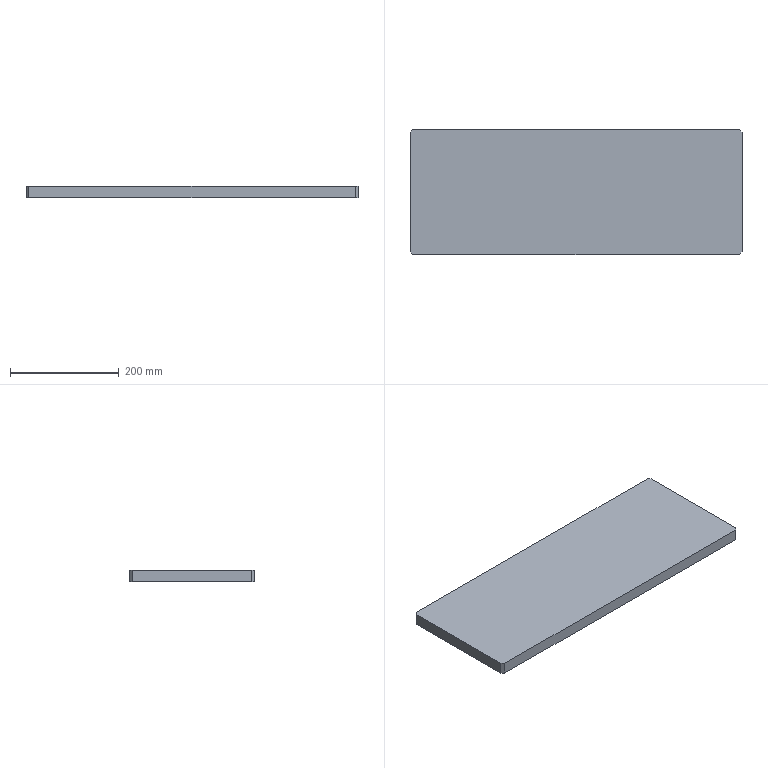Part | SolidWorks | features Chamfer 1, Extrusion 1 | 1 solid | 10 faces | box 610 x 230 x 22 mm | volume 3085500 mm3 | plane 10
STEP:
#1=CARTESIAN_POINT('',(558.381,212.028,22.));
#2=VERTEX_POINT('',#1);
#3=CARTESIAN_POINT('',(-41.619,212.028,22.));
#4=VERTEX_POINT('',#3);
#5=CARTESIAN_POINT('',(-46.619,212.028,22.));
#6=DIRECTION('',(-1.,0.,0.));
#7=VECTOR('',#6,1000.);
#8=LINE('',#5,#7);
#9=EDGE_CURVE('',#2,#4,#8,.T.);
#10=ORIENTED_EDGE('',*,*,#9,.F.);
#11=CARTESIAN_POINT('',(558.381,212.028,0.));
#12=VERTEX_POINT('',#11);
#13=CARTESIAN_POINT('',(558.381,212.028,22.));
#14=DIRECTION('',(0.,0.,-1.));
#15=VECTOR('',#14,1000.);
#16=LINE('',#13,#15);
#17=EDGE_CURVE('',#2,#12,#16,.T.);
#18=ORIENTED_EDGE('',*,*,#17,.T.);
#19=CARTESIAN_POINT('',(-41.619,212.028,0.));
#20=VERTEX_POINT('',#19);
#21=CARTESIAN_POINT('',(-46.619,212.028,0.));
#22=DIRECTION('',(-1.,0.,0.));
#23=VECTOR('',#22,1000.);
#24=LINE('',#21,#23);
#25=EDGE_CURVE('',#12,#20,#24,.T.);
#26=ORIENTED_EDGE('',*,*,#25,.T.);
#27=CARTESIAN_POINT('',(-41.619,212.028,22.));
#28=DIRECTION('',(0.,0.,1.));
#29=VECTOR('',#28,1000.);
#30=LINE('',#27,#29);
#31=EDGE_CURVE('',#20,#4,#30,.T.);
#32=ORIENTED_EDGE('',*,*,#31,.T.);
#33=EDGE_LOOP('',(#10,#18,#26,#32));
#34=FACE_OUTER_BOUND('',#33,.T.);
#35=CARTESIAN_POINT('',(-46.619,212.028,22.));
#36=DIRECTION('',(0.,-1.,0.));
#37=DIRECTION('',(0.,0.,-1.));
#38=AXIS2_PLACEMENT_3D('',#35,#36,#37);
#39=PLANE('',#38);
#40=ADVANCED_FACE('',(#34),#39,.F.);
#41=CARTESIAN_POINT('',(-46.619,207.028,0.));
#42=VERTEX_POINT('',#41);
#43=CARTESIAN_POINT('',(-46.619,-12.972,0.));
#44=VERTEX_POINT('',#43);
#45=CARTESIAN_POINT('',(-46.619,212.028,0.));
#46=DIRECTION('',(0.,-1.,0.));
#47=VECTOR('',#46,1000.);
#48=LINE('',#45,#47);
#49=EDGE_CURVE('',#42,#44,#48,.T.);
#50=ORIENTED_EDGE('',*,*,#49,.T.);
#51=CARTESIAN_POINT('',(-46.619,-12.972,22.));
#52=VERTEX_POINT('',#51);
#53=CARTESIAN_POINT('',(-46.619,-12.972,22.));
#54=DIRECTION('',(0.,0.,1.));
#55=VECTOR('',#54,1000.);
#56=LINE('',#53,#55);
#57=EDGE_CURVE('',#44,#52,#56,.T.);
#58=ORIENTED_EDGE('',*,*,#57,.T.);
#59=CARTESIAN_POINT('',(-46.619,207.028,22.));
#60=VERTEX_POINT('',#59);
#61=CARTESIAN_POINT('',(-46.619,212.028,22.));
#62=DIRECTION('',(0.,-1.,0.));
#63=VECTOR('',#62,1000.);
#64=LINE('',#61,#63);
#65=EDGE_CURVE('',#60,#52,#64,.T.);
#66=ORIENTED_EDGE('',*,*,#65,.F.);
#67=CARTESIAN_POINT('',(-46.619,207.028,22.));
#68=DIRECTION('',(0.,0.,-1.));
#69=VECTOR('',#68,1000.);
#70=LINE('',#67,#69);
#71=EDGE_CURVE('',#60,#42,#70,.T.);
#72=ORIENTED_EDGE('',*,*,#71,.T.);
#73=EDGE_LOOP('',(#50,#58,#66,#72));
#74=FACE_OUTER_BOUND('',#73,.T.);
#75=CARTESIAN_POINT('',(-46.619,212.028,22.));
#76=DIRECTION('',(1.,0.,0.));
#77=DIRECTION('',(0.,1.,0.));
#78=AXIS2_PLACEMENT_3D('',#75,#76,#77);
#79=PLANE('',#78);
#80=ADVANCED_FACE('',(#74),#79,.F.);
#81=CARTESIAN_POINT('',(-41.619,-17.972,0.));
#82=VERTEX_POINT('',#81);
#83=CARTESIAN_POINT('',(558.381,-17.972,0.));
#84=VERTEX_POINT('',#83);
#85=CARTESIAN_POINT('',(563.381,-17.972,0.));
#86=DIRECTION('',(1.,0.,0.));
#87=VECTOR('',#86,1000.);
#88=LINE('',#85,#87);
#89=EDGE_CURVE('',#82,#84,#88,.T.);
#90=ORIENTED_EDGE('',*,*,#89,.T.);
#91=CARTESIAN_POINT('',(558.381,-17.972,22.));
#92=VERTEX_POINT('',#91);
#93=CARTESIAN_POINT('',(558.381,-17.972,22.));
#94=DIRECTION('',(0.,0.,1.));
#95=VECTOR('',#94,1000.);
#96=LINE('',#93,#95);
#97=EDGE_CURVE('',#84,#92,#96,.T.);
#98=ORIENTED_EDGE('',*,*,#97,.T.);
#99=CARTESIAN_POINT('',(-41.619,-17.972,22.));
#100=VERTEX_POINT('',#99);
#101=CARTESIAN_POINT('',(563.381,-17.972,22.));
#102=DIRECTION('',(1.,0.,0.));
#103=VECTOR('',#102,1000.);
#104=LINE('',#101,#103);
#105=EDGE_CURVE('',#100,#92,#104,.T.);
#106=ORIENTED_EDGE('',*,*,#105,.F.);
#107=CARTESIAN_POINT('',(-41.619,-17.972,22.));
#108=DIRECTION('',(0.,0.,-1.));
#109=VECTOR('',#108,1000.);
#110=LINE('',#107,#109);
#111=EDGE_CURVE('',#100,#82,#110,.T.);
#112=ORIENTED_EDGE('',*,*,#111,.T.);
#113=EDGE_LOOP('',(#90,#98,#106,#112));
#114=FACE_OUTER_BOUND('',#113,.T.);
#115=CARTESIAN_POINT('',(563.381,-17.972,22.));
#116=DIRECTION('',(0.,1.,0.));
#117=DIRECTION('',(-1.,0.,0.));
#118=AXIS2_PLACEMENT_3D('',#115,#116,#117);
#119=PLANE('',#118);
#120=ADVANCED_FACE('',(#114),#119,.F.);
#121=CARTESIAN_POINT('',(563.381,-12.972,22.));
#122=VERTEX_POINT('',#121);
#123=CARTESIAN_POINT('',(563.381,207.028,22.));
#124=VERTEX_POINT('',#123);
#125=CARTESIAN_POINT('',(563.381,212.028,22.));
#126=DIRECTION('',(0.,1.,0.));
#127=VECTOR('',#126,1000.);
#128=LINE('',#125,#127);
#129=EDGE_CURVE('',#122,#124,#128,.T.);
#130=ORIENTED_EDGE('',*,*,#129,.F.);
#131=CARTESIAN_POINT('',(563.381,-12.972,0.));
#132=VERTEX_POINT('',#131);
#133=CARTESIAN_POINT('',(563.381,-12.972,22.));
#134=DIRECTION('',(0.,0.,-1.));
#135=VECTOR('',#134,1000.);
#136=LINE('',#133,#135);
#137=EDGE_CURVE('',#122,#132,#136,.T.);
#138=ORIENTED_EDGE('',*,*,#137,.T.);
#139=CARTESIAN_POINT('',(563.381,207.028,0.));
#140=VERTEX_POINT('',#139);
#141=CARTESIAN_POINT('',(563.381,212.028,0.));
#142=DIRECTION('',(0.,1.,0.));
#143=VECTOR('',#142,1000.);
#144=LINE('',#141,#143);
#145=EDGE_CURVE('',#132,#140,#144,.T.);
#146=ORIENTED_EDGE('',*,*,#145,.T.);
#147=CARTESIAN_POINT('',(563.381,207.028,22.));
#148=DIRECTION('',(0.,0.,1.));
#149=VECTOR('',#148,1000.);
#150=LINE('',#147,#149);
#151=EDGE_CURVE('',#140,#124,#150,.T.);
#152=ORIENTED_EDGE('',*,*,#151,.T.);
#153=EDGE_LOOP('',(#130,#138,#146,#152));
#154=FACE_OUTER_BOUND('',#153,.T.);
#155=CARTESIAN_POINT('',(563.381,212.028,22.));
#156=DIRECTION('',(-1.,0.,0.));
#157=DIRECTION('',(0.,0.,1.));
#158=AXIS2_PLACEMENT_3D('',#155,#156,#157);
#159=PLANE('',#158);
#160=ADVANCED_FACE('',(#154),#159,.F.);
#161=ORIENTED_EDGE('',*,*,#105,.T.);
#162=CARTESIAN_POINT('',(563.381,-12.972,22.));
#163=DIRECTION('',(0.7071,0.7071,0.));
#164=VECTOR('',#163,1000.);
#165=LINE('',#162,#164);
#166=EDGE_CURVE('',#92,#122,#165,.T.);
#167=ORIENTED_EDGE('',*,*,#166,.T.);
#168=ORIENTED_EDGE('',*,*,#129,.T.);
#169=CARTESIAN_POINT('',(558.381,212.028,22.));
#170=DIRECTION('',(-0.7071,0.7071,0.));
#171=VECTOR('',#170,1000.);
#172=LINE('',#169,#171);
#173=EDGE_CURVE('',#124,#2,#172,.T.);
#174=ORIENTED_EDGE('',*,*,#173,.T.);
#175=ORIENTED_EDGE('',*,*,#9,.T.);
#176=CARTESIAN_POINT('',(-46.619,207.028,22.));
#177=DIRECTION('',(-0.7071,-0.7071,0.));
#178=VECTOR('',#177,1000.);
#179=LINE('',#176,#178);
#180=EDGE_CURVE('',#4,#60,#179,.T.);
#181=ORIENTED_EDGE('',*,*,#180,.T.);
#182=ORIENTED_EDGE('',*,*,#65,.T.);
#183=CARTESIAN_POINT('',(-41.619,-17.972,22.));
#184=DIRECTION('',(0.7071,-0.7071,0.));
#185=VECTOR('',#184,1000.);
#186=LINE('',#183,#185);
#187=EDGE_CURVE('',#52,#100,#186,.T.);
#188=ORIENTED_EDGE('',*,*,#187,.T.);
#189=EDGE_LOOP('',(#161,#167,#168,#174,#175,#181,#182,#188));
#190=FACE_OUTER_BOUND('',#189,.T.);
#191=CARTESIAN_POINT('',(0.,0.,22.));
#192=DIRECTION('',(0.,0.,-1.));
#193=DIRECTION('',(-1.,0.,0.));
#194=AXIS2_PLACEMENT_3D('',#191,#192,#193);
#195=PLANE('',#194);
#196=ADVANCED_FACE('',(#190),#195,.F.);
#197=ORIENTED_EDGE('',*,*,#145,.F.);
#198=CARTESIAN_POINT('',(288.177,-288.177,0.));
#199=DIRECTION('',(-0.7071,-0.7071,0.));
#200=VECTOR('',#199,1000.);
#201=LINE('',#198,#200);
#202=EDGE_CURVE('',#132,#84,#201,.T.);
#203=ORIENTED_EDGE('',*,*,#202,.T.);
#204=ORIENTED_EDGE('',*,*,#89,.F.);
#205=CARTESIAN_POINT('',(-29.795,-29.795,0.));
#206=DIRECTION('',(-0.7071,0.7071,0.));
#207=VECTOR('',#206,1000.);
#208=LINE('',#205,#207);
#209=EDGE_CURVE('',#82,#44,#208,.T.);
#210=ORIENTED_EDGE('',*,*,#209,.T.);
#211=ORIENTED_EDGE('',*,*,#49,.F.);
#212=CARTESIAN_POINT('',(-126.823,126.823,0.));
#213=DIRECTION('',(0.7071,0.7071,0.));
#214=VECTOR('',#213,1000.);
#215=LINE('',#212,#214);
#216=EDGE_CURVE('',#42,#20,#215,.T.);
#217=ORIENTED_EDGE('',*,*,#216,.T.);
#218=ORIENTED_EDGE('',*,*,#25,.F.);
#219=CARTESIAN_POINT('',(385.205,385.205,0.));
#220=DIRECTION('',(0.7071,-0.7071,0.));
#221=VECTOR('',#220,1000.);
#222=LINE('',#219,#221);
#223=EDGE_CURVE('',#12,#140,#222,.T.);
#224=ORIENTED_EDGE('',*,*,#223,.T.);
#225=EDGE_LOOP('',(#197,#203,#204,#210,#211,#217,#218,#224));
#226=FACE_OUTER_BOUND('',#225,.T.);
#227=CARTESIAN_POINT('',(0.,0.,0.));
#228=DIRECTION('',(0.,0.,-1.));
#229=DIRECTION('',(-1.,0.,0.));
#230=AXIS2_PLACEMENT_3D('',#227,#228,#229);
#231=PLANE('',#230);
#232=ADVANCED_FACE('',(#226),#231,.T.);
#233=ORIENTED_EDGE('',*,*,#166,.F.);
#234=ORIENTED_EDGE('',*,*,#97,.F.);
#235=ORIENTED_EDGE('',*,*,#202,.F.);
#236=ORIENTED_EDGE('',*,*,#137,.F.);
#237=EDGE_LOOP('',(#233,#234,#235,#236));
#238=FACE_OUTER_BOUND('',#237,.T.);
#239=CARTESIAN_POINT('',(563.381,-12.972,22.));
#240=DIRECTION('',(-0.7071,0.7071,0.));
#241=DIRECTION('',(0.,0.,-1.));
#242=AXIS2_PLACEMENT_3D('',#239,#240,#241);
#243=PLANE('',#242);
#244=ADVANCED_FACE('',(#238),#243,.F.);
#245=ORIENTED_EDGE('',*,*,#173,.F.);
#246=ORIENTED_EDGE('',*,*,#151,.F.);
#247=ORIENTED_EDGE('',*,*,#223,.F.);
#248=ORIENTED_EDGE('',*,*,#17,.F.);
#249=EDGE_LOOP('',(#245,#246,#247,#248));
#250=FACE_OUTER_BOUND('',#249,.T.);
#251=CARTESIAN_POINT('',(558.381,212.028,22.));
#252=DIRECTION('',(-0.7071,-0.7071,0.));
#253=DIRECTION('',(0.,0.,-1.));
#254=AXIS2_PLACEMENT_3D('',#251,#252,#253);
#255=PLANE('',#254);
#256=ADVANCED_FACE('',(#250),#255,.F.);
#257=ORIENTED_EDGE('',*,*,#187,.F.);
#258=ORIENTED_EDGE('',*,*,#57,.F.);
#259=ORIENTED_EDGE('',*,*,#209,.F.);
#260=ORIENTED_EDGE('',*,*,#111,.F.);
#261=EDGE_LOOP('',(#257,#258,#259,#260));
#262=FACE_OUTER_BOUND('',#261,.T.);
#263=CARTESIAN_POINT('',(-41.619,-17.972,22.));
#264=DIRECTION('',(0.7071,0.7071,0.));
#265=DIRECTION('',(0.,0.,-1.));
#266=AXIS2_PLACEMENT_3D('',#263,#264,#265);
#267=PLANE('',#266);
#268=ADVANCED_FACE('',(#262),#267,.F.);
#269=ORIENTED_EDGE('',*,*,#180,.F.);
#270=ORIENTED_EDGE('',*,*,#31,.F.);
#271=ORIENTED_EDGE('',*,*,#216,.F.);
#272=ORIENTED_EDGE('',*,*,#71,.F.);
#273=EDGE_LOOP('',(#269,#270,#271,#272));
#274=FACE_OUTER_BOUND('',#273,.T.);
#275=CARTESIAN_POINT('',(-46.619,207.028,22.));
#276=DIRECTION('',(0.7071,-0.7071,0.));
#277=DIRECTION('',(0.,0.,-1.));
#278=AXIS2_PLACEMENT_3D('',#275,#276,#277);
#279=PLANE('',#278);
#280=ADVANCED_FACE('',(#274),#279,.F.);
#281=CLOSED_SHELL('',(#40,#80,#120,#160,#196,#232,#244,#256,#268,#280));
#282=MANIFOLD_SOLID_BREP('',#281);
#283=CARTESIAN_POINT('',(0.,0.,0.));
#284=DIRECTION('',(0.,0.,1.));
#285=DIRECTION('',(1.,0.,0.));
#286=AXIS2_PLACEMENT_3D('',#283,#284,#285);
#287=(LENGTH_UNIT()NAMED_UNIT(*)SI_UNIT(.MILLI.,.METRE.));
#288=UNCERTAINTY_MEASURE_WITH_UNIT(LENGTH_MEASURE(0.00001),#287,'','');
#289=(NAMED_UNIT(*)PLANE_ANGLE_UNIT()SI_UNIT($,.RADIAN.));
#290=(NAMED_UNIT(*)SI_UNIT($,.STERADIAN.)SOLID_ANGLE_UNIT());
#291=(GEOMETRIC_REPRESENTATION_CONTEXT(3)GLOBAL_UNCERTAINTY_ASSIGNED_CONTEXT((#288))GLOBAL_UNIT_ASSIGNED_CONTEXT((#287,#289,#290))REPRESENTATION_CONTEXT('',''));
#292=ADVANCED_BREP_SHAPE_REPRESENTATION('',(#282,#286),#291);